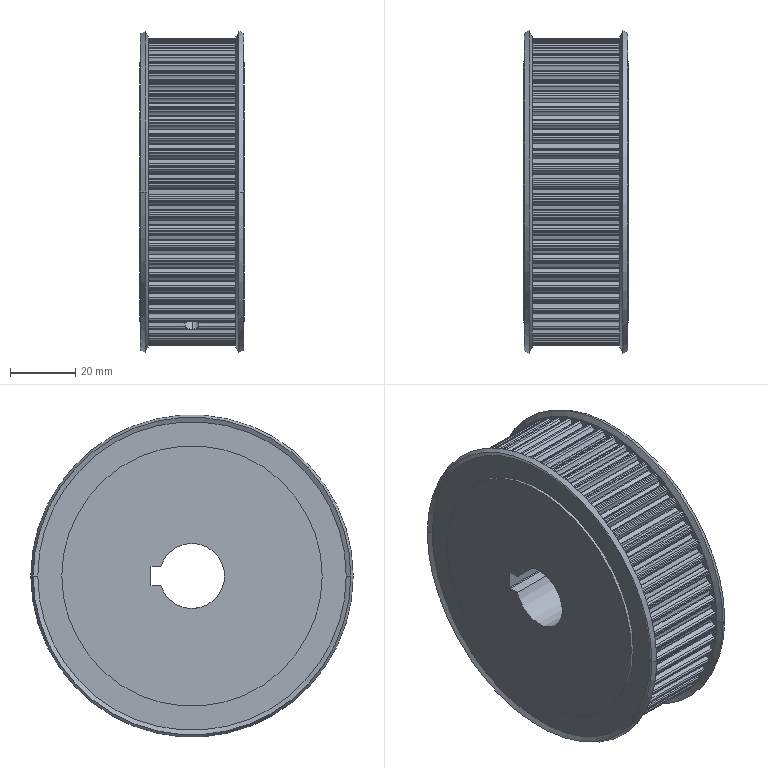Part | NX | 1 solid | 555 faces | box 32 x 99 x 99 mm | volume 203465 mm3 | cylinder 534 | cone 12 | plane 9 | commonest cylinder face diameters 0.5 x124 1.1 x124 6.55 x124 94.53 x88 90.99 x63 4.917 x4